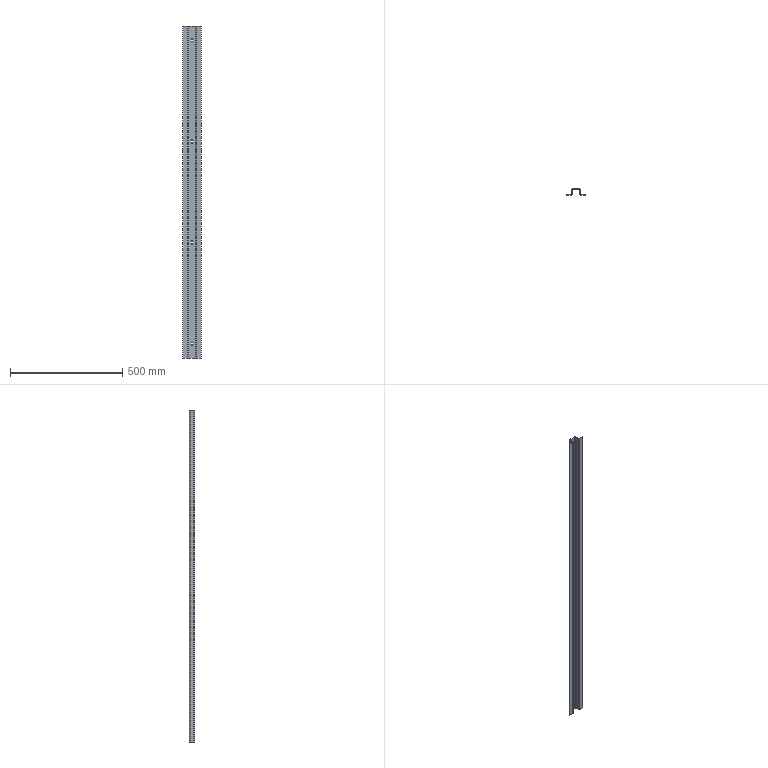Part | STEP file | SYL_0392D6J1SYL0380DJ1006_2_5-1 | 1 solid | 62 faces | box 84 x 25 x 1478 mm | volume 368355 mm3 | plane 38 | cylinder 24 | commonest cylinder face diameters 7 x16 4 x4 8 x4